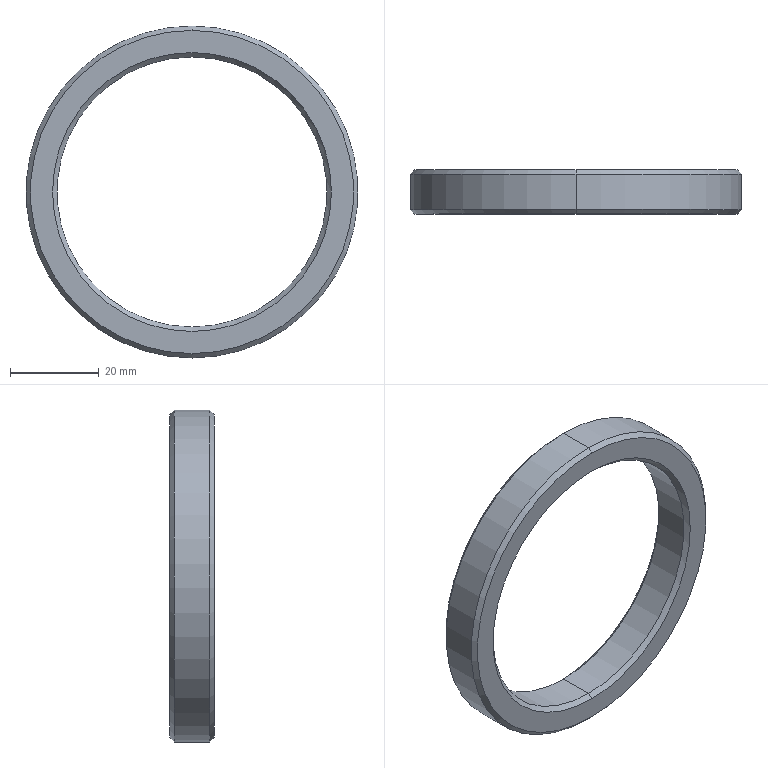Part | SolidWorks | features Chamfer 1, Extrusion 1 | 1 solid | 14 faces | box 75 x 10 x 75 mm | volume 14527 mm3 | cone 8 | cylinder 4 | plane 2 | commonest cylinder face diameters 61 x2 75 x2
STEP:
#1=CARTESIAN_POINT('',(0.,1.,30.5));
#2=VERTEX_POINT('',#1);
#3=CARTESIAN_POINT('',(0.,1.,-30.5));
#4=VERTEX_POINT('',#3);
#5=CARTESIAN_POINT('',(0.,1.,0.));
#6=DIRECTION('',(0.,-1.,0.));
#7=DIRECTION('',(0.,0.,1.));
#8=AXIS2_PLACEMENT_3D('',#5,#6,#7);
#9=CIRCLE('',#8,30.5);
#10=EDGE_CURVE('',#2,#4,#9,.T.);
#11=ORIENTED_EDGE('',*,*,#10,.F.);
#12=CARTESIAN_POINT('',(0.,0.,31.5));
#13=VERTEX_POINT('',#12);
#14=CARTESIAN_POINT('',(0.,0.,31.5));
#15=DIRECTION('',(0.,-0.7071,0.7071));
#16=VECTOR('',#15,1000.);
#17=LINE('',#14,#16);
#18=EDGE_CURVE('',#2,#13,#17,.T.);
#19=ORIENTED_EDGE('',*,*,#18,.T.);
#20=CARTESIAN_POINT('',(0.,0.,-31.5));
#21=VERTEX_POINT('',#20);
#22=CARTESIAN_POINT('',(0.,0.,0.));
#23=DIRECTION('',(0.,1.,0.));
#24=DIRECTION('',(0.,0.,1.));
#25=AXIS2_PLACEMENT_3D('',#22,#23,#24);
#26=CIRCLE('',#25,31.5);
#27=EDGE_CURVE('',#21,#13,#26,.T.);
#28=ORIENTED_EDGE('',*,*,#27,.F.);
#29=CARTESIAN_POINT('',(0.,0.,-31.5));
#30=DIRECTION('',(0.,-0.7071,-0.7071));
#31=VECTOR('',#30,1000.);
#32=LINE('',#29,#31);
#33=EDGE_CURVE('',#4,#21,#32,.T.);
#34=ORIENTED_EDGE('',*,*,#33,.F.);
#35=EDGE_LOOP('',(#11,#19,#28,#34));
#36=FACE_OUTER_BOUND('',#35,.T.);
#37=CARTESIAN_POINT('',(0.,0.,0.));
#38=DIRECTION('',(0.,-1.,0.));
#39=DIRECTION('',(0.,0.,-1.));
#40=AXIS2_PLACEMENT_3D('',#37,#38,#39);
#41=CONICAL_SURFACE('',#40,31.5,0.7854);
#42=ADVANCED_FACE('',(#36),#41,.F.);
#43=CARTESIAN_POINT('',(0.,9.,-30.5));
#44=VERTEX_POINT('',#43);
#45=CARTESIAN_POINT('',(0.,9.,30.5));
#46=VERTEX_POINT('',#45);
#47=CARTESIAN_POINT('',(0.,9.,0.));
#48=DIRECTION('',(0.,1.,0.));
#49=DIRECTION('',(0.,0.,1.));
#50=AXIS2_PLACEMENT_3D('',#47,#48,#49);
#51=CIRCLE('',#50,30.5);
#52=EDGE_CURVE('',#44,#46,#51,.T.);
#53=ORIENTED_EDGE('',*,*,#52,.F.);
#54=CARTESIAN_POINT('',(0.,10.,-31.5));
#55=VERTEX_POINT('',#54);
#56=CARTESIAN_POINT('',(0.,9.,-30.5));
#57=DIRECTION('',(0.,0.7071,-0.7071));
#58=VECTOR('',#57,1000.);
#59=LINE('',#56,#58);
#60=EDGE_CURVE('',#44,#55,#59,.T.);
#61=ORIENTED_EDGE('',*,*,#60,.T.);
#62=CARTESIAN_POINT('',(0.,10.,31.5));
#63=VERTEX_POINT('',#62);
#64=CARTESIAN_POINT('',(0.,10.,0.));
#65=DIRECTION('',(0.,-1.,0.));
#66=DIRECTION('',(0.,0.,1.));
#67=AXIS2_PLACEMENT_3D('',#64,#65,#66);
#68=CIRCLE('',#67,31.5);
#69=EDGE_CURVE('',#63,#55,#68,.T.);
#70=ORIENTED_EDGE('',*,*,#69,.F.);
#71=CARTESIAN_POINT('',(0.,9.,30.5));
#72=DIRECTION('',(0.,0.7071,0.7071));
#73=VECTOR('',#72,1000.);
#74=LINE('',#71,#73);
#75=EDGE_CURVE('',#46,#63,#74,.T.);
#76=ORIENTED_EDGE('',*,*,#75,.F.);
#77=EDGE_LOOP('',(#53,#61,#70,#76));
#78=FACE_OUTER_BOUND('',#77,.T.);
#79=CARTESIAN_POINT('',(0.,9.,0.));
#80=DIRECTION('',(0.,1.,0.));
#81=DIRECTION('',(0.,0.,1.));
#82=AXIS2_PLACEMENT_3D('',#79,#80,#81);
#83=CONICAL_SURFACE('',#82,30.5,0.7854);
#84=ADVANCED_FACE('',(#78),#83,.F.);
#85=CARTESIAN_POINT('',(0.,0.,-36.5));
#86=VERTEX_POINT('',#85);
#87=CARTESIAN_POINT('',(0.,0.,36.5));
#88=VERTEX_POINT('',#87);
#89=CARTESIAN_POINT('',(0.,0.,0.));
#90=DIRECTION('',(0.,-1.,0.));
#91=DIRECTION('',(0.,0.,1.));
#92=AXIS2_PLACEMENT_3D('',#89,#90,#91);
#93=CIRCLE('',#92,36.5);
#94=EDGE_CURVE('',#86,#88,#93,.T.);
#95=ORIENTED_EDGE('',*,*,#94,.F.);
#96=CARTESIAN_POINT('',(0.,1.,-37.5));
#97=VERTEX_POINT('',#96);
#98=CARTESIAN_POINT('',(0.,1.,-37.5));
#99=DIRECTION('',(0.,0.7071,-0.7071));
#100=VECTOR('',#99,1000.);
#101=LINE('',#98,#100);
#102=EDGE_CURVE('',#86,#97,#101,.T.);
#103=ORIENTED_EDGE('',*,*,#102,.T.);
#104=CARTESIAN_POINT('',(0.,1.,37.5));
#105=VERTEX_POINT('',#104);
#106=CARTESIAN_POINT('',(0.,1.,0.));
#107=DIRECTION('',(0.,1.,0.));
#108=DIRECTION('',(0.,0.,1.));
#109=AXIS2_PLACEMENT_3D('',#106,#107,#108);
#110=CIRCLE('',#109,37.5);
#111=EDGE_CURVE('',#105,#97,#110,.T.);
#112=ORIENTED_EDGE('',*,*,#111,.F.);
#113=CARTESIAN_POINT('',(0.,1.,37.5));
#114=DIRECTION('',(0.,0.7071,0.7071));
#115=VECTOR('',#114,1000.);
#116=LINE('',#113,#115);
#117=EDGE_CURVE('',#88,#105,#116,.T.);
#118=ORIENTED_EDGE('',*,*,#117,.F.);
#119=EDGE_LOOP('',(#95,#103,#112,#118));
#120=FACE_OUTER_BOUND('',#119,.T.);
#121=CARTESIAN_POINT('',(0.,1.,0.));
#122=DIRECTION('',(0.,1.,0.));
#123=DIRECTION('',(0.,0.,1.));
#124=AXIS2_PLACEMENT_3D('',#121,#122,#123);
#125=CONICAL_SURFACE('',#124,37.5,0.7854);
#126=ADVANCED_FACE('',(#120),#125,.T.);
#127=CARTESIAN_POINT('',(0.,10.,36.5));
#128=VERTEX_POINT('',#127);
#129=CARTESIAN_POINT('',(0.,10.,-36.5));
#130=VERTEX_POINT('',#129);
#131=CARTESIAN_POINT('',(0.,10.,0.));
#132=DIRECTION('',(0.,1.,0.));
#133=DIRECTION('',(0.,0.,1.));
#134=AXIS2_PLACEMENT_3D('',#131,#132,#133);
#135=CIRCLE('',#134,36.5);
#136=EDGE_CURVE('',#128,#130,#135,.T.);
#137=ORIENTED_EDGE('',*,*,#136,.F.);
#138=CARTESIAN_POINT('',(0.,9.,37.5));
#139=VERTEX_POINT('',#138);
#140=CARTESIAN_POINT('',(0.,10.,36.5));
#141=DIRECTION('',(0.,-0.7071,0.7071));
#142=VECTOR('',#141,1000.);
#143=LINE('',#140,#142);
#144=EDGE_CURVE('',#128,#139,#143,.T.);
#145=ORIENTED_EDGE('',*,*,#144,.T.);
#146=CARTESIAN_POINT('',(0.,9.,-37.5));
#147=VERTEX_POINT('',#146);
#148=CARTESIAN_POINT('',(0.,9.,0.));
#149=DIRECTION('',(0.,-1.,0.));
#150=DIRECTION('',(0.,0.,1.));
#151=AXIS2_PLACEMENT_3D('',#148,#149,#150);
#152=CIRCLE('',#151,37.5);
#153=EDGE_CURVE('',#147,#139,#152,.T.);
#154=ORIENTED_EDGE('',*,*,#153,.F.);
#155=CARTESIAN_POINT('',(0.,10.,-36.5));
#156=DIRECTION('',(0.,-0.7071,-0.7071));
#157=VECTOR('',#156,1000.);
#158=LINE('',#155,#157);
#159=EDGE_CURVE('',#130,#147,#158,.T.);
#160=ORIENTED_EDGE('',*,*,#159,.F.);
#161=EDGE_LOOP('',(#137,#145,#154,#160));
#162=FACE_OUTER_BOUND('',#161,.T.);
#163=CARTESIAN_POINT('',(0.,10.,0.));
#164=DIRECTION('',(0.,-1.,0.));
#165=DIRECTION('',(0.,0.,-1.));
#166=AXIS2_PLACEMENT_3D('',#163,#164,#165);
#167=CONICAL_SURFACE('',#166,36.5,0.7854);
#168=ADVANCED_FACE('',(#162),#167,.T.);
#169=ORIENTED_EDGE('',*,*,#52,.T.);
#170=CARTESIAN_POINT('',(0.,10.,30.5));
#171=DIRECTION('',(0.,-1.,0.));
#172=VECTOR('',#171,1000.);
#173=LINE('',#170,#172);
#174=EDGE_CURVE('',#46,#2,#173,.T.);
#175=ORIENTED_EDGE('',*,*,#174,.T.);
#176=ORIENTED_EDGE('',*,*,#10,.T.);
#177=CARTESIAN_POINT('',(0.,10.,-30.5));
#178=DIRECTION('',(0.,-1.,0.));
#179=VECTOR('',#178,1000.);
#180=LINE('',#177,#179);
#181=EDGE_CURVE('',#44,#4,#180,.T.);
#182=ORIENTED_EDGE('',*,*,#181,.F.);
#183=EDGE_LOOP('',(#169,#175,#176,#182));
#184=FACE_OUTER_BOUND('',#183,.T.);
#185=CARTESIAN_POINT('',(0.,10.,0.));
#186=DIRECTION('',(0.,-1.,0.));
#187=DIRECTION('',(0.,0.,-1.));
#188=AXIS2_PLACEMENT_3D('',#185,#186,#187);
#189=CYLINDRICAL_SURFACE('',#188,30.5);
#190=ADVANCED_FACE('',(#184),#189,.F.);
#191=ORIENTED_EDGE('',*,*,#153,.T.);
#192=CARTESIAN_POINT('',(0.,10.,37.5));
#193=DIRECTION('',(0.,-1.,0.));
#194=VECTOR('',#193,1000.);
#195=LINE('',#192,#194);
#196=EDGE_CURVE('',#139,#105,#195,.T.);
#197=ORIENTED_EDGE('',*,*,#196,.T.);
#198=ORIENTED_EDGE('',*,*,#111,.T.);
#199=CARTESIAN_POINT('',(0.,10.,-37.5));
#200=DIRECTION('',(0.,-1.,0.));
#201=VECTOR('',#200,1000.);
#202=LINE('',#199,#201);
#203=EDGE_CURVE('',#147,#97,#202,.T.);
#204=ORIENTED_EDGE('',*,*,#203,.F.);
#205=EDGE_LOOP('',(#191,#197,#198,#204));
#206=FACE_OUTER_BOUND('',#205,.T.);
#207=CARTESIAN_POINT('',(0.,10.,0.));
#208=DIRECTION('',(0.,-1.,0.));
#209=DIRECTION('',(0.,0.,-1.));
#210=AXIS2_PLACEMENT_3D('',#207,#208,#209);
#211=CYLINDRICAL_SURFACE('',#210,37.5);
#212=ADVANCED_FACE('',(#206),#211,.T.);
#213=CARTESIAN_POINT('',(0.,10.,0.));
#214=DIRECTION('',(0.,1.,0.));
#215=DIRECTION('',(0.,0.,1.));
#216=AXIS2_PLACEMENT_3D('',#213,#214,#215);
#217=CIRCLE('',#216,36.5);
#218=EDGE_CURVE('',#130,#128,#217,.T.);
#219=ORIENTED_EDGE('',*,*,#218,.T.);
#220=ORIENTED_EDGE('',*,*,#136,.T.);
#221=EDGE_LOOP('',(#219,#220));
#222=FACE_OUTER_BOUND('',#221,.T.);
#223=ORIENTED_EDGE('',*,*,#69,.T.);
#224=CARTESIAN_POINT('',(0.,10.,0.));
#225=DIRECTION('',(0.,-1.,0.));
#226=DIRECTION('',(0.,0.,1.));
#227=AXIS2_PLACEMENT_3D('',#224,#225,#226);
#228=CIRCLE('',#227,31.5);
#229=EDGE_CURVE('',#55,#63,#228,.T.);
#230=ORIENTED_EDGE('',*,*,#229,.T.);
#231=EDGE_LOOP('',(#223,#230));
#232=FACE_BOUND('',#231,.T.);
#233=CARTESIAN_POINT('',(0.,10.,0.));
#234=DIRECTION('',(0.,1.,0.));
#235=DIRECTION('',(0.,0.,1.));
#236=AXIS2_PLACEMENT_3D('',#233,#234,#235);
#237=PLANE('',#236);
#238=ADVANCED_FACE('',(#222,#232),#237,.T.);
#239=CARTESIAN_POINT('',(0.,0.,0.));
#240=DIRECTION('',(0.,-1.,0.));
#241=DIRECTION('',(0.,0.,1.));
#242=AXIS2_PLACEMENT_3D('',#239,#240,#241);
#243=CIRCLE('',#242,36.5);
#244=EDGE_CURVE('',#88,#86,#243,.T.);
#245=ORIENTED_EDGE('',*,*,#244,.T.);
#246=ORIENTED_EDGE('',*,*,#94,.T.);
#247=EDGE_LOOP('',(#245,#246));
#248=FACE_OUTER_BOUND('',#247,.T.);
#249=ORIENTED_EDGE('',*,*,#27,.T.);
#250=CARTESIAN_POINT('',(0.,0.,0.));
#251=DIRECTION('',(0.,1.,0.));
#252=DIRECTION('',(0.,0.,1.));
#253=AXIS2_PLACEMENT_3D('',#250,#251,#252);
#254=CIRCLE('',#253,31.5);
#255=EDGE_CURVE('',#13,#21,#254,.T.);
#256=ORIENTED_EDGE('',*,*,#255,.T.);
#257=EDGE_LOOP('',(#249,#256));
#258=FACE_BOUND('',#257,.T.);
#259=CARTESIAN_POINT('',(0.,0.,0.));
#260=DIRECTION('',(0.,1.,0.));
#261=DIRECTION('',(0.,0.,1.));
#262=AXIS2_PLACEMENT_3D('',#259,#260,#261);
#263=PLANE('',#262);
#264=ADVANCED_FACE('',(#248,#258),#263,.F.);
#265=ORIENTED_EDGE('',*,*,#196,.F.);
#266=CARTESIAN_POINT('',(0.,9.,0.));
#267=DIRECTION('',(0.,-1.,0.));
#268=DIRECTION('',(0.,0.,1.));
#269=AXIS2_PLACEMENT_3D('',#266,#267,#268);
#270=CIRCLE('',#269,37.5);
#271=EDGE_CURVE('',#139,#147,#270,.T.);
#272=ORIENTED_EDGE('',*,*,#271,.T.);
#273=ORIENTED_EDGE('',*,*,#203,.T.);
#274=CARTESIAN_POINT('',(0.,1.,0.));
#275=DIRECTION('',(0.,1.,0.));
#276=DIRECTION('',(0.,0.,1.));
#277=AXIS2_PLACEMENT_3D('',#274,#275,#276);
#278=CIRCLE('',#277,37.5);
#279=EDGE_CURVE('',#97,#105,#278,.T.);
#280=ORIENTED_EDGE('',*,*,#279,.T.);
#281=EDGE_LOOP('',(#265,#272,#273,#280));
#282=FACE_OUTER_BOUND('',#281,.T.);
#283=CARTESIAN_POINT('',(0.,10.,0.));
#284=DIRECTION('',(0.,-1.,0.));
#285=DIRECTION('',(0.,0.,-1.));
#286=AXIS2_PLACEMENT_3D('',#283,#284,#285);
#287=CYLINDRICAL_SURFACE('',#286,37.5);
#288=ADVANCED_FACE('',(#282),#287,.T.);
#289=ORIENTED_EDGE('',*,*,#174,.F.);
#290=CARTESIAN_POINT('',(0.,9.,0.));
#291=DIRECTION('',(0.,1.,0.));
#292=DIRECTION('',(0.,0.,1.));
#293=AXIS2_PLACEMENT_3D('',#290,#291,#292);
#294=CIRCLE('',#293,30.5);
#295=EDGE_CURVE('',#46,#44,#294,.T.);
#296=ORIENTED_EDGE('',*,*,#295,.T.);
#297=ORIENTED_EDGE('',*,*,#181,.T.);
#298=CARTESIAN_POINT('',(0.,1.,0.));
#299=DIRECTION('',(0.,-1.,0.));
#300=DIRECTION('',(0.,0.,1.));
#301=AXIS2_PLACEMENT_3D('',#298,#299,#300);
#302=CIRCLE('',#301,30.5);
#303=EDGE_CURVE('',#4,#2,#302,.T.);
#304=ORIENTED_EDGE('',*,*,#303,.T.);
#305=EDGE_LOOP('',(#289,#296,#297,#304));
#306=FACE_OUTER_BOUND('',#305,.T.);
#307=CARTESIAN_POINT('',(0.,10.,0.));
#308=DIRECTION('',(0.,-1.,0.));
#309=DIRECTION('',(0.,0.,-1.));
#310=AXIS2_PLACEMENT_3D('',#307,#308,#309);
#311=CYLINDRICAL_SURFACE('',#310,30.5);
#312=ADVANCED_FACE('',(#306),#311,.F.);
#313=ORIENTED_EDGE('',*,*,#144,.F.);
#314=ORIENTED_EDGE('',*,*,#218,.F.);
#315=ORIENTED_EDGE('',*,*,#159,.T.);
#316=ORIENTED_EDGE('',*,*,#271,.F.);
#317=EDGE_LOOP('',(#313,#314,#315,#316));
#318=FACE_OUTER_BOUND('',#317,.T.);
#319=CARTESIAN_POINT('',(0.,10.,0.));
#320=DIRECTION('',(0.,-1.,0.));
#321=DIRECTION('',(0.,0.,-1.));
#322=AXIS2_PLACEMENT_3D('',#319,#320,#321);
#323=CONICAL_SURFACE('',#322,36.5,0.7854);
#324=ADVANCED_FACE('',(#318),#323,.T.);
#325=ORIENTED_EDGE('',*,*,#102,.F.);
#326=ORIENTED_EDGE('',*,*,#244,.F.);
#327=ORIENTED_EDGE('',*,*,#117,.T.);
#328=ORIENTED_EDGE('',*,*,#279,.F.);
#329=EDGE_LOOP('',(#325,#326,#327,#328));
#330=FACE_OUTER_BOUND('',#329,.T.);
#331=CARTESIAN_POINT('',(0.,1.,0.));
#332=DIRECTION('',(0.,1.,0.));
#333=DIRECTION('',(0.,0.,1.));
#334=AXIS2_PLACEMENT_3D('',#331,#332,#333);
#335=CONICAL_SURFACE('',#334,37.5,0.7854);
#336=ADVANCED_FACE('',(#330),#335,.T.);
#337=ORIENTED_EDGE('',*,*,#60,.F.);
#338=ORIENTED_EDGE('',*,*,#295,.F.);
#339=ORIENTED_EDGE('',*,*,#75,.T.);
#340=ORIENTED_EDGE('',*,*,#229,.F.);
#341=EDGE_LOOP('',(#337,#338,#339,#340));
#342=FACE_OUTER_BOUND('',#341,.T.);
#343=CARTESIAN_POINT('',(0.,9.,0.));
#344=DIRECTION('',(0.,1.,0.));
#345=DIRECTION('',(0.,0.,1.));
#346=AXIS2_PLACEMENT_3D('',#343,#344,#345);
#347=CONICAL_SURFACE('',#346,30.5,0.7854);
#348=ADVANCED_FACE('',(#342),#347,.F.);
#349=ORIENTED_EDGE('',*,*,#18,.F.);
#350=ORIENTED_EDGE('',*,*,#303,.F.);
#351=ORIENTED_EDGE('',*,*,#33,.T.);
#352=ORIENTED_EDGE('',*,*,#255,.F.);
#353=EDGE_LOOP('',(#349,#350,#351,#352));
#354=FACE_OUTER_BOUND('',#353,.T.);
#355=CARTESIAN_POINT('',(0.,0.,0.));
#356=DIRECTION('',(0.,-1.,0.));
#357=DIRECTION('',(0.,0.,-1.));
#358=AXIS2_PLACEMENT_3D('',#355,#356,#357);
#359=CONICAL_SURFACE('',#358,31.5,0.7854);
#360=ADVANCED_FACE('',(#354),#359,.F.);
#361=CLOSED_SHELL('',(#42,#84,#126,#168,#190,#212,#238,#264,#288,#312,#324,#336,#348,#360));
#362=MANIFOLD_SOLID_BREP('',#361);
#363=CARTESIAN_POINT('',(0.,0.,0.));
#364=DIRECTION('',(0.,0.,1.));
#365=DIRECTION('',(1.,0.,0.));
#366=AXIS2_PLACEMENT_3D('',#363,#364,#365);
#367=(LENGTH_UNIT()NAMED_UNIT(*)SI_UNIT(.MILLI.,.METRE.));
#368=UNCERTAINTY_MEASURE_WITH_UNIT(LENGTH_MEASURE(0.00001),#367,'','');
#369=(NAMED_UNIT(*)PLANE_ANGLE_UNIT()SI_UNIT($,.RADIAN.));
#370=(NAMED_UNIT(*)SI_UNIT($,.STERADIAN.)SOLID_ANGLE_UNIT());
#371=(GEOMETRIC_REPRESENTATION_CONTEXT(3)GLOBAL_UNCERTAINTY_ASSIGNED_CONTEXT((#368))GLOBAL_UNIT_ASSIGNED_CONTEXT((#367,#369,#370))REPRESENTATION_CONTEXT('',''));
#372=ADVANCED_BREP_SHAPE_REPRESENTATION('',(#362,#366),#371);